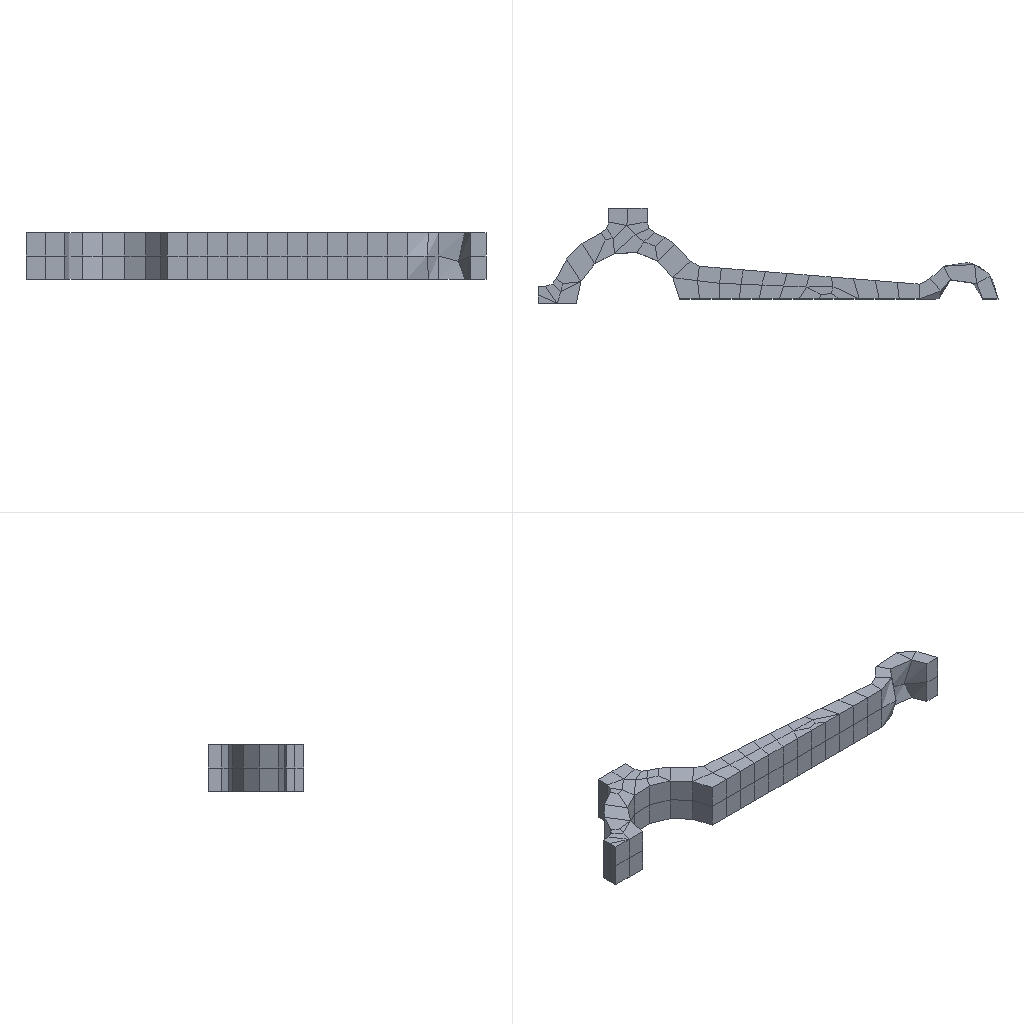Simulation study | ansys workbench
Set-up summary:
category,name,step,type,value,unit,region
solver,ansys_workbench
units,mm-N-s-tonne (MPa),,stated,"/units,MPA"
analysis,LS1,,static
load_step,LS1,LS1,static,nsubst=1; time=1
mesh,nodes,,,773
mesh,elements,,,144
element_type,SOLID186,,,96
element_type,SURF154,,,48
material,Structural Steel,,E,200000,tonne s^-2 mm^-1
material,Structural Steel,,nu,0.3
material,Structural Steel,,density,7.85e-09,tonne mm^-3
material,Structural Steel,,conductivity,60.5,tonne mm s^-3 C^-1
material,Structural Steel,,specific_heat,4.34e+08,mm^2 s^-2 C^-1
material,Structural Steel,,cte,1.2e-05,C^-1
material,Structural Steel,,permeability,10000
material,Structural Steel,,resistivity,0.00017,ohm mm
load,Define Force Using Surface Effect Elements,LS1,surface-effect pres face 3,-0.2145,,SURF154 #2
bc,Fixed Supports,model,fixed,[dofs=ALL],,_FIXEDSU
named_set,_FIXEDSU,,node,90
Ansys APDL input file, long lists of numbers shortened:
/batch
/config,noeldb,1     ! force off writing results to database
*get,_wallstrt,active,,time,wall
! ANSYS input file written by Workbench version 2022 R1
! File used for geometry attach:
/title,wbnew--____ (A5)
! ****** Begin Custom Load Command Snippet ******
/COM, ACT Extensions:
/COM,     LSDYNA, 2021.1
/COM,
! ****** End   Custom Load Command Snippet ******
*DIM,_wb_ProjectScratch_dir,string,248
_wb_ProjectScratch_dir(1) = ''
*DIM,_wb_SolverFiles_dir,string,248
_wb_SolverFiles_dir(1) = ''
*DIM,_wb_userfiles_dir,string,248
_wb_userfiles_dir(1) = ''
/com,--- Data in consistent NMM units. See Solving Units in the help system for more information.
/units,MPA
/nopr
/wb,file,start              !  signify a WB generated input file
/prep7
! Turn off shape checking because checks already performed inside WB mesher.
! See help system for more information.
SHPP,OFF,,NOWARN
/nolist
etcon,set             ! allow ANSYS to choose best KEYOP's for 180x elements, resets any applicable keyopt to MAPDL defaults
/com,*********** Nodes for the whole assembly ***********
nblock,3,,850
(1i9,3e20.9e3)
        1     8.391578362E+01     3.870075414E+00     0.000000000E+00
! (772 more lines like these left out)
-1
/wb,elem,start            !  set before creation of elements
/com,*********** Elements for Body 1 "__-FreeParts|__-__1" ***********
et,1,186
keyo,1,2,1          ! set full integration on SOLID186
eblock,19,solid,,96
(19i9)
        1        1        1        1        0        0        0        0       20        0        1        1        2        3        4       34       33       32       31
! (191 more lines like these left out)
-1
/wb,elem,end               !  done creating elements
/com,*********** Send User Defined Coordinate System(s) ***********
csys,0
toffst,273.15,  ! Temperature offset from absolute zero
/com,*********** Set Reference Temperature ***********
tref,22.
/wb,mat,start              !  starting to send materials
/com,*********** Send Materials ***********
Temperature = 'TEMP' ! Temperature
MP,DENS,1,7.85e-09,	! tonne mm^-3
MP,ALPX,1,1.2e-05,	! C^-1
MP,C,1,434000000,	! mm^2 s^-2 C^-1
MP,KXX,1,60.5,	! tonne mm s^-3 C^-1
MP,RSVX,1,0.00017,	! ohm mm
MP,EX,1,200000,	! tonne s^-2 mm^-1
MP,NUXY,1,0.3,
MP,MURX,1,10000,
/wb,mat,end                !  done sending materials
!************************* Model Summary ********************
!__-FreeParts|__-__1,	结构钢,	matid,	1
!************************* End Model Summary ********************
! get the diagonal of the bounding box. Needed later for other things
*get,_xmin,node,,mnloc,x
*get,_ymin,node,,mnloc,y
*get,_zmin,node,,mnloc,z
*get,_xmax,node,,mxloc,x
*get,_ymax,node,,mxloc,y
*get,_zmax,node,,mxloc,z
_ASMDIAG=(_xmax-_xmin)*(_xmax-_xmin)+(_ymax-_ymin)*(_ymax-_ymin)+(_zmax-_zmin)*(_zmax-_zmin)
_ASMDIAG=SQRT(_ASMDIAG)
/wb,contact,start          !  starting to send contact
/wb,contact,end            !  done creating contacts
/golist
/wb,load,start             !  starting to send loads
/com,*********** Fixed Supports ***********
CMBLOCK,_FIXEDSU,NODE,       90
(8i10)
        82        83        84        85        98        99       100       101
! (11 more lines like these left out)
cmsel,s,_FIXEDSU
d,all,all
nsel,all
/com,*********** Define Force Using Surface Effect Elements ***********
local,12,0,0.,0.,0.,0.,0.,0.
csys,0
et,2,154
eblock,10,,,48
(15i9)
      317        2        2        2       12       23      138       24       24      340      343       24      338
! (47 more lines like these left out)
-1
esel,s,type,,2
keyop,2,2,1                ! Apply load in local coordinate system
keyop,2,7,1                ! Use original area so load is constant in large deformation
esel,all
/gst,on,on
fini
*get,_numnode,node,0,count
*get,_numelem,elem,0,count
*get, _MAXELEMNUM, elem, 0, NUM, MAX
*get, _MAXNODENUM, node, 0, NUM, MAX
*get, _MAXELEMTYPE, etyp, 0, NUM, MAX
*get, _MAXREALCONST, real, 0, NUM, MAX
/go
/wb,load,end               !  done creating loads
/com,--- Number of total nodes = %_numnode%
/com,--- Number of contact elements = 48
/com,--- Number of spring elements = 0
/com,--- Number of bearing elements = 0
/com,--- Number of solid elements = 96
/com,--- Number of condensed parts = 0
/com,--- Number of total elements = %_numelem%
*get,_wallbsol,active,,time,wall
/com,****************************************************************************
/com,*************************    SOLUTION       ********************************
/com,****************************************************************************
/solu
antype,0                   ! static analysis
_thickRatio=  0     ! Ratio of thick parts in the model
eqsl,sparse,,,,,1
cntr,print,1               ! print out contact info and also make no initial contact an error
dmpoption,emat,no             ! Don't combine emat file for DANSYS
dmpoption,esav,no             ! Don't combine esav file for DANSYS
nldiag,cont,iter           ! print out contact info each equilibrium iteration
rescontrol,,none                 ! Do not keep any restart files
/com,****************************************************
/com,******************* SOLVE FOR LS 1 OF 1 ****************
esel,s,type,,2
nsle
sfe,all,1,pres,1,0.
sfe,all,2,pres,1,0.
sfe,all,3,pres,1,-0.2145
nsel,all
esel,all
/nopr
/gopr
nsub,1,1,1
time,1.
outres,erase
outres,all,none
outres,nsol,all,
outres,rsol,all
outres,eangl,all
outres,etmp,all
outres,veng,all
outres,strs,all,
outres,epel,all,
outres,eppl,all,
outres,cont,all,
! *********** WB SOLVE COMMAND ***********
! check interactive state
*get,ANSINTER_,active,,int
*if,ANSINTER_,ne,0,then
/eof
*endif
solve
/com *************** Write FE CONNECTORS *********
CEWRITE,file,ce,,INTE
/com,****************************************************
/com,*************** FINISHED SOLVE FOR LS 1 *************
*get,_wallasol,active,,time,wall
/nopr
*get,_numnode,node,0,count
*get,_numelem,elem,0,count
*get, _MAXELEMNUM, elem, 0, NUM, MAX
*get, _MAXNODENUM, node, 0, NUM, MAX,,,INTERNAL
*get, _MAXELEMTYPE, etyp, 0, NUM, MAX
*get, _MAXREALCONST, real, 0, NUM, MAX
/gopr
/post1
xmlo,ENCODING,ISO-8859-1
xmlo,parm
/xml,parm,xml
fini
/gopr
*get,_walldone,active,,time,wall
_preptime=(_wallbsol-_wallstrt)*3600
_solvtime=(_wallasol-_wallbsol)*3600
_posttime=(_walldone-_wallasol)*3600
_totaltim=(_walldone-_wallstrt)*3600
*get,_dlbratio,active,0,solu,dlbr
*get,_combtime,active,0,solu,comb
*get,_ssmode,active,0,solu,ssmm
*get,_ndofs,active,0,solu,ndof
*get,_sol_end_time,active,0,set,time
*if,_sol_end_time,eq,1.,then
/fclean				!clean distributed files
*endif
/com,--- Total number of nodes = %_numnode%
/com,--- Total number of elements = %_numelem%
/com,--- Element load balance ratio = %_dlbratio%
/com,--- Time to combine distributed files = %_combtime%
/com,--- Sparse memory mode = %_ssmode%
/com,--- Number of DOF = %_ndofs%
/wb,file,end               ! done with WB generated input
Results summary:
result,analyses[0].index,,,1
result,analyses[0].system,,,SYS
result,analyses[0].deck,,,deck.dat
result,analyses[0].solve_status,,,completed
result,analyses[0].analysis_type,,,static
result,analyses[0].physics,,,mechanical
result,analyses[0].unit_system,,,"NMM: mm, ton, N, s, mV, mA, degC"
result,analyses[0].n_sets,,,1
result,analyses[0].load_steps[0].set,set=1,,1
result,analyses[0].load_steps[0].time_or_freq,set=1,,1
result,analyses[0].load_steps[0].max_displacement_magnitude,set=1,,0.001038
result,analyses[0].load_steps[0].max_von_mises_nodal,set=1,,5.326
result,analyses[0].load_steps[0].reaction_force_sum_xyz[1],set=1,,8.02913e-13
result,analyses[0].load_steps[0].reaction_force_sum_xyz[2],set=1,,-2.74625e-12
result,analyses[0].load_steps[0].reaction_force_sum_xyz[3],set=1,,500